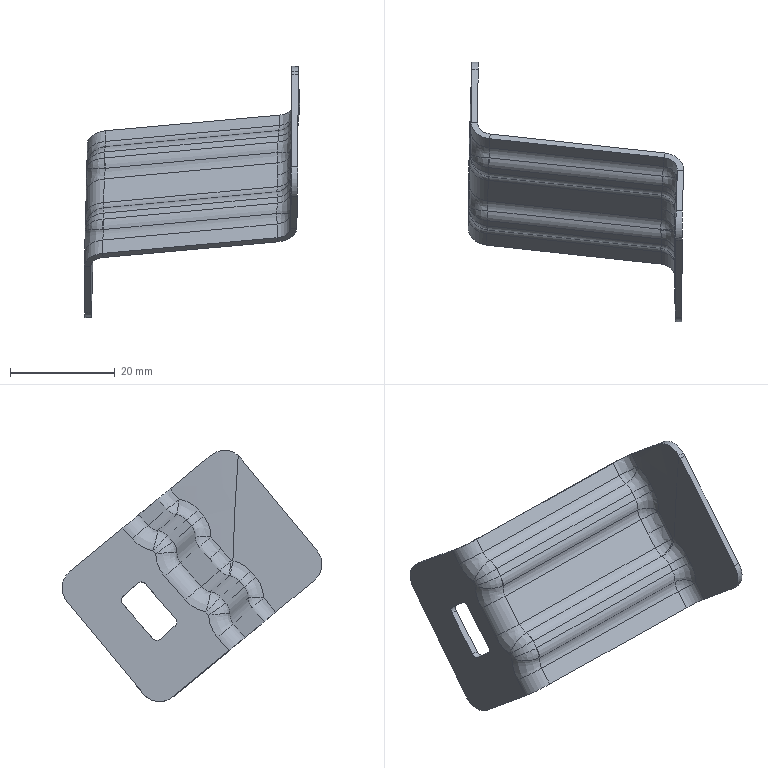Part | 1 solid | 121 faces | box 41.123 x 49.636 x 48.023 mm | volume 2762 mm3 | spline 51 | cylinder 34 | plane 25 | sphere 8 | other 3 | commonest cylinder face diameters 6 x10 8.4 x6 5.6 x5 8 x5 2 x4 3.6 x4